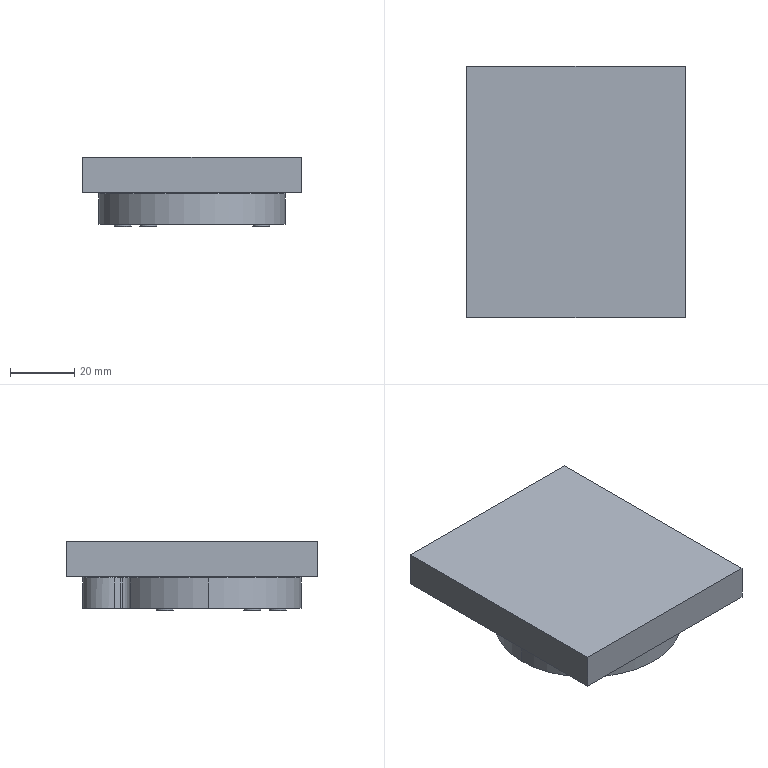NC program | NX | posted with a generic post | part box 68 x 78.27 x 21.8 mm
Lines 2834 to 3556 of 10371:
(CAVITY_MILL_COPY_COPY_COPY , TOOL : D2)
N5636 T17 M6
N5638 G54
N5640 G17 G0 G90 X1.507 Y24.709 S9500 M3
N5642 G43 Z30. H17
N5644 Z-0.5
N5646 G94 G1 Z-1. F1000.
N5648 G3 X0.772 Y24.654 R1.
N5650 G2 X0.207 Y24.506 R1.5 F2000.
N5652 G1 X-0.012 Y24.116
N5654 X-0.093 Y23.976
N5656 G3 X-0.189 Y23.149 R1.
N5658 G1 Z-0.5
N5660 G0 X1.507 Y24.709 Z-0.7
N5662 G1 Z-1.2 F1000.
N5664 G3 X0.772 Y24.654 R1.
N5666 G2 X0.207 Y24.506 R1.5 F2000.
N5668 G1 X-0.012 Y24.116
N5670 X-0.093 Y23.976
N5672 G3 X-0.189 Y23.149 R1.
N5674 G1 Z-0.7
N5676 G0 X1.507 Y24.709 Z-0.9
N5678 G1 Z-1.4 F1000.
N5680 G3 X0.772 Y24.654 R1.
N5682 G2 X0.207 Y24.506 R1.5 F2000.
N5684 G1 X-0.012 Y24.116
N5686 X-0.093 Y23.976
N5688 G3 X-0.189 Y23.149 R1.
N5690 G1 Z-0.9
N5692 G0 X1.507 Y24.709 Z-1.1
N5694 G1 Z-1.6 F1000.
N5696 G3 X0.772 Y24.654 R1.
N5698 G2 X0.207 Y24.506 R1.5 F2000.
N5700 G1 X-0.012 Y24.116
N5702 X-0.093 Y23.976
N5704 G3 X-0.189 Y23.149 R1.
N5706 G1 Z-1.1
N5708 G0 X1.507 Y24.709 Z-1.3
N5710 G1 Z-1.8 F1000.
N5712 G3 X0.772 Y24.654 R1.
N5714 G2 X0.207 Y24.506 R1.5 F2000.
N5716 G1 X-0.012 Y24.116
N5718 X-0.093 Y23.976
N5720 G3 X-0.189 Y23.149 R1.
N5722 G1 Z-1.3
N5724 G0 X1.507 Y24.709 Z-1.5
N5726 G1 Z-2. F1000.
N5728 G3 X0.772 Y24.654 R1.
N5730 G2 X0.207 Y24.506 R1.5 F2000.
N5732 G1 X-0.012 Y24.116
N5734 X-0.093 Y23.976
N5736 G3 X-0.189 Y23.149 R1.
N5738 G1 Z-1.5
N5740 G0 X1.507 Y24.709 Z-1.7
N5742 G1 Z-2.2 F1000.
N5744 G3 X0.772 Y24.654 R1.
N5746 G2 X0.207 Y24.506 R1.5 F2000.
N5748 G1 X-0.012 Y24.116
N5750 X-0.093 Y23.976
N5752 G3 X-0.189 Y23.149 R1.
N5754 G1 Z-1.7
N5756 G0 X1.507 Y24.709 Z-1.9
N5758 G1 Z-2.4 F1000.
N5760 G3 X0.772 Y24.654 R1.
N5762 G2 X0.207 Y24.506 R1.5 F2000.
N5764 G1 X-0.012 Y24.116
N5766 X-0.093 Y23.976
N5768 G3 X-0.189 Y23.149 R1.
N5770 G1 Z-1.9
N5772 G0 X1.507 Y24.709 Z-2.1
N5774 G1 Z-2.6 F1000.
N5776 G3 X0.772 Y24.654 R1.
N5778 G2 X0.207 Y24.506 R1.5 F2000.
N5780 G1 X-0.012 Y24.116
N5782 X-0.093 Y23.976
N5784 G3 X-0.189 Y23.149 R1.
N5786 G1 Z-2.1
N5788 G0 X1.507 Y24.709 Z-2.3
N5790 G1 Z-2.8 F1000.
N5792 G3 X0.772 Y24.654 R1.
N5794 G2 X0.207 Y24.506 R1.5 F2000.
N5796 G1 X-0.012 Y24.116
N5798 X-0.093 Y23.976
N5800 G3 X-0.189 Y23.149 R1.
N5802 G1 Z-2.3
N5804 G0 X1.507 Y24.709 Z-2.5
N5806 G1 Z-3. F1000.
N5808 G3 X0.772 Y24.654 R1.
N5810 G2 X0.207 Y24.506 R1.5 F2000.
N5812 G1 X-0.012 Y24.116
N5814 X-0.093 Y23.976
N5816 G3 X-0.189 Y23.149 R1.
N5818 G1 Z-2.5
N5820 G0 X1.507 Y24.709 Z-2.7
N5822 G1 Z-3.2 F1000.
N5824 G3 X0.772 Y24.654 R1.
N5826 G2 X0.207 Y24.506 R1.5 F2000.
N5828 G1 X-0.012 Y24.116
N5830 X-0.093 Y23.976
N5832 G3 X-0.189 Y23.149 R1.
N5834 G1 Z-2.7
N5836 G0 X1.507 Y24.709 Z-2.9
N5838 G1 Z-3.4 F1000.
N5840 G3 X0.772 Y24.654 R1.
N5842 G2 X0.207 Y24.506 R1.5 F2000.
N5844 G1 X-0.012 Y24.116
N5846 X-0.093 Y23.976
N5848 G3 X-0.189 Y23.149 R1.
N5850 G1 Z-2.9
N5852 G0 X1.507 Y24.709 Z-3.1
N5854 G1 Z-3.6 F1000.
N5856 G3 X0.772 Y24.654 R1.
N5858 G2 X0.207 Y24.506 R1.5 F2000.
N5860 G1 X-0.012 Y24.116
N5862 X-0.093 Y23.976
N5864 G3 X-0.189 Y23.149 R1.
N5866 G1 Z-3.1
N5868 G0 X1.507 Y24.709 Z-3.3
N5870 G1 Z-3.8 F1000.
N5872 G3 X0.772 Y24.654 R1.
N5874 G2 X0.207 Y24.506 R1.5 F2000.
N5876 G1 X-0.012 Y24.116
N5878 X-0.093 Y23.976
N5880 G3 X-0.189 Y23.149 R1.
N5882 G1 Z-3.3
N5884 G0 X1.507 Y24.709 Z-3.5
N5886 G1 Z-4. F1000.
N5888 G3 X0.772 Y24.654 R1.
N5890 G2 X0.207 Y24.506 R1.5 F2000.
N5892 G1 X-0.012 Y24.116
N5894 X-0.093 Y23.976
N5896 G3 X-0.189 Y23.149 R1.
N5898 G1 Z-3.5
N5900 G0 X1.507 Y24.709 Z-3.7
N5902 G1 Z-4.2 F1000.
N5904 G3 X0.772 Y24.654 R1.
N5906 G2 X0.207 Y24.506 R1.5 F2000.
N5908 G1 X-0.012 Y24.116
N5910 X-0.093 Y23.976
N5912 G3 X-0.189 Y23.149 R1.
N5914 G1 Z-3.7
N5916 G0 X1.507 Y24.709 Z-3.9
N5918 G1 Z-4.4 F1000.
N5920 G3 X0.772 Y24.654 R1.
N5922 G2 X0.207 Y24.506 R1.5 F2000.
N5924 G1 X-0.012 Y24.116
N5926 X-0.093 Y23.976
N5928 G3 X-0.189 Y23.149 R1.
N5930 G1 Z-3.9
N5932 G0 X1.507 Y24.709 Z-4.1
N5934 G1 Z-4.6 F1000.
N5936 G3 X0.772 Y24.654 R1.
N5938 G2 X0.207 Y24.506 R1.5 F2000.
N5940 G1 X-0.012 Y24.116
N5942 X-0.093 Y23.976
N5944 G3 X-0.189 Y23.149 R1.
N5946 G1 Z-4.1
N5948 G0 X1.507 Y24.709 Z-4.3
N5950 G1 Z-4.8 F1000.
N5952 G3 X0.772 Y24.654 R1.
N5954 G2 X0.207 Y24.506 R1.5 F2000.
N5956 G1 X-0.012 Y24.116
N5958 X-0.093 Y23.976
N5960 G3 X-0.189 Y23.149 R1.
N5962 G1 Z-4.3
N5964 G0 X1.507 Y24.709 Z-4.5
N5966 G1 Z-5. F1000.
N5968 G3 X0.772 Y24.654 R1.
N5970 G2 X0.207 Y24.506 R1.5 F2000.
N5972 G1 X-0.012 Y24.116
N5974 X-0.093 Y23.976
N5976 G3 X-0.189 Y23.149 R1.
N5978 G1 Z-4.5
N5980 G0 X1.507 Y24.709 Z-4.7
N5982 G1 Z-5.2 F1000.
N5984 G3 X0.772 Y24.654 R1.
N5986 G2 X0.207 Y24.506 R1.5 F2000.
N5988 G1 X-0.012 Y24.116
N5990 X-0.093 Y23.976
N5992 G3 X-0.189 Y23.149 R1.
N5994 G1 Z-4.7
N5996 G0 X1.507 Y24.709 Z-4.9
N5998 G1 Z-5.4 F1000.
N6000 G3 X0.772 Y24.654 R1.
N6002 G2 X0.207 Y24.506 R1.5 F2000.
N6004 G1 X-0.012 Y24.116
N6006 X-0.093 Y23.976
N6008 G3 X-0.189 Y23.149 R1.
N6010 G1 Z-4.9
N6012 G0 X1.507 Y24.709 Z-5.1
N6014 G1 Z-5.6 F1000.
N6016 G3 X0.772 Y24.654 R1.
N6018 G2 X0.207 Y24.506 R1.5 F2000.
N6020 G1 X-0.012 Y24.116
N6022 X-0.093 Y23.976
N6024 G3 X-0.189 Y23.149 R1.
N6026 G1 Z-5.1
N6028 G0 X1.507 Y24.709 Z-5.3
N6030 G1 Z-5.8 F1000.
N6032 G3 X0.772 Y24.654 R1.
N6034 G2 X0.207 Y24.506 R1.5 F2000.
N6036 G1 X-0.012 Y24.116
N6038 X-0.093 Y23.976
N6040 G3 X-0.189 Y23.149 R1.
N6042 G1 Z-5.3
N6044 G0 X1.507 Y24.709 Z-5.5
N6046 G1 Z-6. F1000.
N6048 G3 X0.772 Y24.654 R1.
N6050 G2 X0.207 Y24.506 R1.5 F2000.
N6052 G1 X-0.012 Y24.116
N6054 X-0.093 Y23.976
N6056 G3 X-0.189 Y23.149 R1.
N6058 G1 Z-5.5
N6060 G0 X1.507 Y24.709 Z-5.7
N6062 G1 Z-6.2 F1000.
N6064 G3 X0.772 Y24.654 R1.
N6066 G2 X0.207 Y24.506 R1.5 F2000.
N6068 G1 X-0.012 Y24.116
N6070 X-0.093 Y23.976
N6072 G3 X-0.189 Y23.149 R1.
N6074 G1 Z-5.7
N6076 G0 X1.507 Y24.709 Z-5.9
N6078 G1 Z-6.4 F1000.
N6080 G3 X0.772 Y24.654 R1.
N6082 G2 X0.207 Y24.506 R1.5 F2000.
N6084 G1 X-0.012 Y24.116
N6086 X-0.093 Y23.976
N6088 G3 X-0.189 Y23.149 R1.
N6090 G1 Z-5.9
N6092 G0 X1.507 Y24.709 Z-6.1
N6094 G1 Z-6.6 F1000.
N6096 G3 X0.772 Y24.654 R1.
N6098 G2 X0.207 Y24.506 R1.5 F2000.
N6100 G1 X-0.012 Y24.116
N6102 X-0.093 Y23.976
N6104 G3 X-0.189 Y23.149 R1.
N6106 G1 Z-6.1
N6108 G0 X1.507 Y24.709 Z-6.3
N6110 G1 Z-6.8 F1000.
N6112 G3 X0.772 Y24.654 R1.
N6114 G2 X0.207 Y24.506 R1.5 F2000.
N6116 G1 X-0.012 Y24.116
N6118 X-0.093 Y23.976
N6120 G3 X-0.189 Y23.149 R1.
N6122 G1 Z-6.3
N6124 G0 X1.507 Y24.709 Z-6.5
N6126 G1 Z-7. F1000.
N6128 G3 X0.772 Y24.654 R1.
N6130 G2 X0.207 Y24.506 R1.5 F2000.
N6132 G1 X-0.012 Y24.116
N6134 X-0.093 Y23.976
N6136 G3 X-0.189 Y23.149 R1.
N6138 G1 Z-6.5
N6140 G0 X1.507 Y24.709 Z-6.7
N6142 G1 Z-7.2 F1000.
N6144 G3 X0.772 Y24.654 R1.
N6146 G2 X0.207 Y24.506 R1.5 F2000.
N6148 G1 X-0.012 Y24.116
N6150 X-0.093 Y23.976
N6152 G3 X-0.189 Y23.149 R1.
N6154 G1 Z-6.7
N6156 G0 X1.507 Y24.709 Z-6.9
N6158 G1 Z-7.4 F1000.
N6160 G3 X0.772 Y24.654 R1.
N6162 G2 X0.207 Y24.506 R1.5 F2000.
N6164 G1 X-0.012 Y24.116
N6166 X-0.093 Y23.976
N6168 G3 X-0.189 Y23.149 R1.
N6170 G1 Z-6.9
N6172 G0 X1.507 Y24.709 Z-7.1
N6174 G1 Z-7.6 F1000.
N6176 G3 X0.772 Y24.654 R1.
N6178 G2 X0.207 Y24.506 R1.5 F2000.
N6180 G1 X-0.012 Y24.116
N6182 X-0.093 Y23.976
N6184 G3 X-0.189 Y23.149 R1.
N6186 G1 Z-7.1
N6188 G0 X1.507 Y24.709 Z-7.3
N6190 G1 Z-7.8 F1000.
N6192 G3 X0.772 Y24.654 R1.
N6194 G2 X0.207 Y24.506 R1.5 F2000.
N6196 G1 X-0.012 Y24.116
N6198 X-0.093 Y23.976
N6200 G3 X-0.189 Y23.149 R1.
N6202 G1 Z-7.3
N6204 G0 X1.507 Y24.709 Z-7.5
N6206 G1 Z-8. F1000.
N6208 G3 X0.772 Y24.654 R1.
N6210 G2 X0.207 Y24.506 R1.5 F2000.
N6212 G1 X-0.012 Y24.116
N6214 X-0.093 Y23.976
N6216 G3 X-0.189 Y23.149 R1.
N6218 G1 Z-7.5
N6220 G0 X1.507 Y24.709 Z-7.7
N6222 G1 Z-8.2 F1000.
N6224 G3 X0.772 Y24.654 R1.
N6226 G2 X0.207 Y24.506 R1.5 F2000.
N6228 G1 X-0.012 Y24.116
N6230 X-0.093 Y23.976
N6232 G3 X-0.189 Y23.149 R1.
N6234 G1 Z-7.7
N6236 G0 X1.507 Y24.709 Z-7.9
N6238 G1 Z-8.4 F1000.
N6240 G3 X0.772 Y24.654 R1.
N6242 G2 X0.207 Y24.506 R1.5 F2000.
N6244 G1 X-0.012 Y24.116
N6246 X-0.093 Y23.976
N6248 G3 X-0.189 Y23.149 R1.
N6250 G1 Z-7.9
N6252 G0 X1.507 Y24.709 Z-8.1
N6254 G1 Z-8.6 F1000.
N6256 G3 X0.772 Y24.654 R1.
N6258 G2 X0.207 Y24.506 R1.5 F2000.
N6260 G1 X-0.012 Y24.116
N6262 X-0.093 Y23.976
N6264 G3 X-0.189 Y23.149 R1.
N6266 G1 Z-8.1
N6268 G0 X1.507 Y24.709 Z-8.3
N6270 G1 Z-8.8 F1000.
N6272 G3 X0.772 Y24.654 R1.
N6274 G2 X0.207 Y24.506 R1.5 F2000.
N6276 G1 X-0.012 Y24.116
N6278 X-0.093 Y23.976
N6280 G3 X-0.189 Y23.149 R1.
N6282 G1 Z-8.3
N6284 G0 X1.764 Y23.744 Z-8.5
N6286 G1 Z-9. F1000.
N6288 G3 X1.071 Y24.31 R1.
N6290 G1 X0.207 Y24.506 F2000.
N6292 X-0.012 Y24.116
N6294 G2 X-0.237 Y23.752 R5.
N6296 G3 X-0.377 Y22.931 R1.
N6298 G1 Z-8.5
N6300 G0 X1.764 Y23.744 Z-8.7
N6302 G1 Z-9.2 F1000.
N6304 G3 X1.071 Y24.31 R1.
N6306 G1 X0.207 Y24.506 F2000.
N6308 X-0.012 Y24.116
N6310 G2 X-0.237 Y23.752 R5.
N6312 G3 X-0.377 Y22.931 R1.
N6314 G1 Z-8.7
N6316 G0 X1.764 Y23.744 Z-8.9
N6318 G1 Z-9.4 F1000.
N6320 G3 X1.071 Y24.31 R1.
N6322 G1 X0.207 Y24.506 F2000.
N6324 X-0.012 Y24.116
N6326 G2 X-0.237 Y23.752 R5.
N6328 G3 X-0.377 Y22.931 R1.
N6330 G1 Z-8.9
N6332 G0 X1.764 Y23.744 Z-9.1
N6334 G1 Z-9.6 F1000.
N6336 G3 X1.071 Y24.31 R1.
N6338 G1 X0.207 Y24.506 F2000.
N6340 X-0.012 Y24.116
N6342 G2 X-0.237 Y23.752 R5.
N6344 G3 X-0.377 Y22.931 R1.
N6346 G1 Z-9.1
N6348 G0 X1.764 Y23.744 Z-9.3
N6350 G1 Z-9.8 F1000.
N6352 G3 X1.071 Y24.31 R1.
N6354 G1 X0.207 Y24.506 F2000.
N6356 X-0.012 Y24.116
N6358 G2 X-0.237 Y23.752 R5.
N6360 G3 X-0.377 Y22.931 R1.
N6362 G1 Z-9.3
N6364 G0 Z-5.8
N6366 X11.299 Y20.207
N6368 Z-8.5
N6370 G1 Z-9. F1000.
N6372 G3 X11.604 Y21.027 R1.
N6374 G2 X11.576 Y21.59 R6. F2000.
N6376 G3 X10.947 Y22.079 R1.
N6378 X10.051 Y21.871 R1.
N6380 G1 Z-8.5
N6382 G0 X11.299 Y20.207 Z-8.7
N6384 G1 Z-9.2 F1000.
N6386 G3 X11.604 Y21.027 R1.
N6388 G2 X11.576 Y21.59 R6. F2000.
N6390 G3 X10.947 Y22.079 R1.
N6392 X10.051 Y21.871 R1.
N6394 G1 Z-8.7
N6396 G0 X11.299 Y20.207 Z-8.9
N6398 G1 Z-9.4 F1000.
N6400 G3 X11.604 Y21.027 R1.
N6402 G2 X11.576 Y21.59 R6. F2000.
N6404 G3 X10.947 Y22.079 R1.
N6406 X10.051 Y21.871 R1.
N6408 G1 Z-8.9
N6410 G0 X11.299 Y20.207 Z-9.1
N6412 G1 Z-9.6 F1000.
N6414 G3 X11.604 Y21.027 R1.
N6416 G2 X11.576 Y21.59 R6. F2000.
N6418 G3 X10.947 Y22.079 R1.
N6420 X10.051 Y21.871 R1.
N6422 G1 Z-9.1
N6424 G0 X11.299 Y20.207 Z-9.3
N6426 G1 Z-9.8 F1000.
N6428 G3 X11.604 Y21.027 R1.
N6430 G2 X11.576 Y21.59 R6. F2000.
N6432 G3 X10.947 Y22.079 R1.
N6434 X10.051 Y21.871 R1.
N6436 G1 Z-9.3
N6438 G0 Z30.
N6440 X-15.708 Y16.332
N6442 Z-0.5
N6444 G1 Z-1. F1000.
N6446 G3 X-16.599 Y16.16 R1.
N6448 X-17.192 Y15.684 R27. F2000.
N6450 G2 X-17.093 Y14.996 R1.5
N6452 G3 X-16.885 Y14.288 R1.
N6454 G1 Z-0.5
N6456 G0 X-15.708 Y16.332 Z-0.7
N6458 G1 Z-1.2 F1000.
N6460 G3 X-16.599 Y16.16 R1.
N6462 X-17.192 Y15.684 R27. F2000.
N6464 G2 X-17.093 Y14.996 R1.5
N6466 G3 X-16.885 Y14.288 R1.
N6468 G1 Z-0.7
N6470 G0 X-15.708 Y16.332 Z-0.9
N6472 G1 Z-1.4 F1000.
N6474 G3 X-16.599 Y16.16 R1.
N6476 X-17.192 Y15.684 R27. F2000.
N6478 G2 X-17.093 Y14.996 R1.5
N6480 G3 X-16.885 Y14.288 R1.
N6482 G1 Z-0.9
N6484 G0 X-15.708 Y16.332 Z-1.1
N6486 G1 Z-1.6 F1000.
N6488 G3 X-16.599 Y16.16 R1.
N6490 X-17.192 Y15.684 R27. F2000.
N6492 G2 X-17.093 Y14.996 R1.5
N6494 G3 X-16.885 Y14.288 R1.
N6496 G1 Z-1.1
N6498 G0 X-15.708 Y16.332 Z-1.3
N6500 G1 Z-1.8 F1000.
N6502 G3 X-16.599 Y16.16 R1.
N6504 X-17.192 Y15.684 R27. F2000.
N6506 G2 X-17.093 Y14.996 R1.5
N6508 G3 X-16.885 Y14.288 R1.
N6510 G1 Z-1.3
N6512 G0 X-15.708 Y16.332 Z-1.5
N6514 G1 Z-2. F1000.
N6516 G3 X-16.599 Y16.16 R1.
N6518 X-17.192 Y15.684 R27. F2000.
N6520 G2 X-17.093 Y14.996 R1.5
N6522 G3 X-16.885 Y14.288 R1.
N6524 G1 Z-1.5
N6526 G0 X-15.708 Y16.332 Z-1.7
N6528 G1 Z-2.2 F1000.
N6530 G3 X-16.599 Y16.16 R1.
N6532 X-17.192 Y15.684 R27. F2000.
N6534 G2 X-17.093 Y14.996 R1.5
N6536 G3 X-16.885 Y14.288 R1.
N6538 G1 Z-1.7
N6540 G0 X-15.708 Y16.332 Z-1.9
N6542 G1 Z-2.4 F1000.
N6544 G3 X-16.599 Y16.16 R1.
N6546 X-17.192 Y15.684 R27. F2000.
N6548 G2 X-17.093 Y14.996 R1.5
N6550 G3 X-16.885 Y14.288 R1.
N6552 G1 Z-1.9
N6554 G0 X-15.708 Y16.332 Z-2.1
N6556 G1 Z-2.6 F1000.
N6558 G3 X-16.599 Y16.16 R1.
N6560 X-17.192 Y15.684 R27. F2000.
N6562 G2 X-17.093 Y14.996 R1.5
N6564 G3 X-16.885 Y14.288 R1.
N6566 G1 Z-2.1
N6568 G0 X-15.708 Y16.332 Z-2.3
N6570 G1 Z-2.8 F1000.
N6572 G3 X-16.599 Y16.16 R1.
N6574 X-17.192 Y15.684 R27. F2000.
N6576 G2 X-17.093 Y14.996 R1.5
N6578 G3 X-16.885 Y14.288 R1.
N6580 G1 Z-2.3
N6582 G0 X-15.708 Y16.332 Z-2.5
N6584 G1 Z-3. F1000.
N6586 G3 X-16.599 Y16.16 R1.
N6588 X-17.192 Y15.684 R27. F2000.
N6590 G2 X-17.093 Y14.996 R1.5
N6592 G3 X-16.885 Y14.288 R1.
N6594 G1 Z-2.5
N6596 G0 X-15.708 Y16.332 Z-2.7
N6598 G1 Z-3.2 F1000.
N6600 G3 X-16.599 Y16.16 R1.
N6602 X-17.192 Y15.684 R27. F2000.
N6604 G2 X-17.093 Y14.996 R1.5
N6606 G3 X-16.885 Y14.288 R1.
N6608 G1 Z-2.7
N6610 G0 X-15.708 Y16.332 Z-2.9
N6612 G1 Z-3.4 F1000.
N6614 G3 X-16.599 Y16.16 R1.
N6616 X-17.192 Y15.684 R27. F2000.
N6618 G2 X-17.093 Y14.996 R1.5
N6620 G3 X-16.885 Y14.288 R1.
N6622 G1 Z-2.9
N6624 G0 X-15.708 Y16.332 Z-3.1
N6626 G1 Z-3.6 F1000.
N6628 G3 X-16.599 Y16.16 R1.
N6630 X-17.192 Y15.684 R27. F2000.
N6632 G2 X-17.093 Y14.996 R1.5
N6634 G3 X-16.885 Y14.288 R1.
N6636 G1 Z-3.1
N6638 G0 X-15.708 Y16.332 Z-3.3
N6640 G1 Z-3.8 F1000.
N6642 G3 X-16.599 Y16.16 R1.
N6644 X-17.192 Y15.684 R27. F2000.
N6646 G2 X-17.093 Y14.996 R1.5
N6648 G3 X-16.885 Y14.288 R1.
N6650 G1 Z-3.3
N6652 G0 X-15.708 Y16.332 Z-3.5
N6654 G1 Z-4. F1000.
N6656 G3 X-16.599 Y16.16 R1.
N6658 X-17.192 Y15.684 R27. F2000.
N6660 G2 X-17.093 Y14.996 R1.5
N6662 G3 X-16.885 Y14.288 R1.
N6664 G1 Z-3.5
N6666 G0 X-15.708 Y16.332 Z-3.7
N6668 G1 Z-4.2 F1000.
N6670 G3 X-16.599 Y16.16 R1.
N6672 X-17.192 Y15.684 R27. F2000.
N6674 G2 X-17.093 Y14.996 R1.5
N6676 G3 X-16.885 Y14.288 R1.
N6678 G1 Z-3.7
N6680 G0 X-15.708 Y16.332 Z-3.9
N6682 G1 Z-4.4 F1000.
N6684 G3 X-16.599 Y16.16 R1.
N6686 X-17.192 Y15.684 R27. F2000.
N6688 G2 X-17.093 Y14.996 R1.5
N6690 G3 X-16.885 Y14.288 R1.
N6692 G1 Z-3.9
N6694 G0 X-15.708 Y16.332 Z-4.1
N6696 G1 Z-4.6 F1000.
N6698 G3 X-16.599 Y16.16 R1.
N6700 X-17.192 Y15.684 R27. F2000.
N6702 G2 X-17.093 Y14.996 R1.5
N6704 G3 X-16.885 Y14.288 R1.
N6706 G1 Z-4.1
N6708 G0 X-15.708 Y16.332 Z-4.3
N6710 G1 Z-4.8 F1000.
N6712 G3 X-16.599 Y16.16 R1.
N6714 X-17.192 Y15.684 R27. F2000.
N6716 G2 X-17.093 Y14.996 R1.5
N6718 G3 X-16.885 Y14.288 R1.
N6720 G1 Z-4.3
N6722 G0 X-15.708 Y16.332 Z-4.5
N6724 G1 Z-5. F1000.
N6726 G3 X-16.599 Y16.16 R1.
N6728 X-17.192 Y15.684 R27. F2000.
N6730 G2 X-17.093 Y14.996 R1.5
N6732 G3 X-16.885 Y14.288 R1.
N6734 G1 Z-4.5
N6736 G0 X-15.708 Y16.332 Z-4.7
N6738 G1 Z-5.2 F1000.
N6740 G3 X-16.599 Y16.16 R1.
N6742 X-17.192 Y15.684 R27. F2000.
N6744 G2 X-17.093 Y14.996 R1.5
N6746 G3 X-16.885 Y14.288 R1.
N6748 G1 Z-4.7
N6750 G0 X-15.708 Y16.332 Z-4.9
N6752 G1 Z-5.4 F1000.
N6754 G3 X-16.599 Y16.16 R1.
N6756 X-17.192 Y15.684 R27. F2000.
N6758 G2 X-17.093 Y14.996 R1.5
N6760 G3 X-16.885 Y14.288 R1.
N6762 G1 Z-4.9
N6764 G0 X-15.708 Y16.332 Z-5.1
N6766 G1 Z-5.6 F1000.
N6768 G3 X-16.599 Y16.16 R1.
N6770 X-17.192 Y15.684 R27. F2000.
N6772 G2 X-17.093 Y14.996 R1.5
N6774 G3 X-16.885 Y14.288 R1.
N6776 G1 Z-5.1
N6778 G0 X-15.708 Y16.332 Z-5.3
N6780 G1 Z-5.8 F1000.
N6782 G3 X-16.599 Y16.16 R1.
N6784 X-17.192 Y15.684 R27. F2000.
N6786 G2 X-17.093 Y14.996 R1.5
N6788 G3 X-16.885 Y14.288 R1.
N6790 G1 Z-5.3
N6792 G0 X-15.708 Y16.332 Z-5.5
N6794 G1 Z-6. F1000.
N6796 G3 X-16.599 Y16.16 R1.
N6798 X-17.192 Y15.684 R27. F2000.
N6800 G2 X-17.093 Y14.996 R1.5
N6802 G3 X-16.885 Y14.288 R1.
N6804 G1 Z-5.5
N6806 G0 X-15.708 Y16.332 Z-5.7
N6808 G1 Z-6.2 F1000.
N6810 G3 X-16.599 Y16.16 R1.
N6812 X-17.192 Y15.684 R27. F2000.
N6814 G2 X-17.093 Y14.996 R1.5
N6816 G3 X-16.885 Y14.288 R1.
N6818 G1 Z-5.7
N6820 G0 X-15.708 Y16.332 Z-5.9
N6822 G1 Z-6.4 F1000.
N6824 G3 X-16.599 Y16.16 R1.
N6826 X-17.192 Y15.684 R27. F2000.
N6828 G2 X-17.093 Y14.996 R1.5
N6830 G3 X-16.885 Y14.288 R1.
N6832 G1 Z-5.9
N6834 G0 X-15.708 Y16.332 Z-6.1
N6836 G1 Z-6.6 F1000.
N6838 G3 X-16.599 Y16.16 R1.
N6840 X-17.192 Y15.684 R27. F2000.
N6842 G2 X-17.093 Y14.996 R1.5
N6844 G3 X-16.885 Y14.288 R1.
N6846 G1 Z-6.1
N6848 G0 X-15.708 Y16.332 Z-6.3
N6850 G1 Z-6.8 F1000.
N6852 G3 X-16.599 Y16.16 R1.
N6854 X-17.192 Y15.684 R27. F2000.
N6856 G2 X-17.093 Y14.996 R1.5
N6858 G3 X-16.885 Y14.288 R1.
N6860 G1 Z-6.3
N6862 G0 X-15.708 Y16.332 Z-6.5
N6864 G1 Z-7. F1000.
N6866 G3 X-16.599 Y16.16 R1.
N6868 X-17.192 Y15.684 R27. F2000.
N6870 G2 X-17.093 Y14.996 R1.5
N6872 G3 X-16.885 Y14.288 R1.
N6874 G1 Z-6.5
N6876 G0 X-15.708 Y16.332 Z-6.7
N6878 G1 Z-7.2 F1000.
N6880 G3 X-16.599 Y16.16 R1.
N6882 X-17.192 Y15.684 R27. F2000.
N6884 G2 X-17.093 Y14.996 R1.5
N6886 G3 X-16.885 Y14.288 R1.
N6888 G1 Z-6.7
N6890 G0 X-15.708 Y16.332 Z-6.9
N6892 G1 Z-7.4 F1000.
N6894 G3 X-16.599 Y16.16 R1.
N6896 X-17.192 Y15.684 R27. F2000.
N6898 G2 X-17.093 Y14.996 R1.5
N6900 G3 X-16.885 Y14.288 R1.
N6902 G1 Z-6.9
N6904 G0 X-15.708 Y16.332 Z-7.1
N6906 G1 Z-7.6 F1000.
N6908 G3 X-16.599 Y16.16 R1.
N6910 X-17.192 Y15.684 R27. F2000.
N6912 G2 X-17.093 Y14.996 R1.5
N6914 G3 X-16.885 Y14.288 R1.
N6916 G1 Z-7.1
N6918 G0 X-15.708 Y16.332 Z-7.3
N6920 G1 Z-7.8 F1000.
N6922 G3 X-16.599 Y16.16 R1.
N6924 X-17.192 Y15.684 R27. F2000.
N6926 G2 X-17.093 Y14.996 R1.5
N6928 G3 X-16.885 Y14.288 R1.
N6930 G1 Z-7.3
N6932 G0 X-15.708 Y16.332 Z-7.5
N6934 G1 Z-8. F1000.
N6936 G3 X-16.599 Y16.16 R1.
N6938 X-17.192 Y15.684 R27. F2000.
N6940 G2 X-17.093 Y14.996 R1.5
N6942 G3 X-16.885 Y14.288 R1.
N6944 G1 Z-7.5
N6946 G0 X-15.708 Y16.332 Z-7.7
N6948 G1 Z-8.2 F1000.
N6950 G3 X-16.599 Y16.16 R1.
N6952 X-17.192 Y15.684 R27. F2000.
N6954 G2 X-17.093 Y14.996 R1.5
N6956 G3 X-16.885 Y14.288 R1.
N6958 G1 Z-7.7
N6960 G0 X-15.708 Y16.332 Z-7.9
N6962 G1 Z-8.4 F1000.
N6964 G3 X-16.599 Y16.16 R1.
N6966 X-17.192 Y15.684 R27. F2000.
N6968 G2 X-17.093 Y14.996 R1.5
N6970 G3 X-16.885 Y14.288 R1.
N6972 G1 Z-7.9
N6974 G0 X-15.708 Y16.332 Z-8.1
N6976 G1 Z-8.6 F1000.
N6978 G3 X-16.599 Y16.16 R1.
N6980 X-17.192 Y15.684 R27. F2000.
N6982 G2 X-17.093 Y14.996 R1.5
N6984 G3 X-16.885 Y14.288 R1.
N6986 G1 Z-8.1
N6988 G0 X-15.708 Y16.332 Z-8.3
N6990 G1 Z-8.8 F1000.
N6992 G3 X-16.599 Y16.16 R1.
N6994 X-17.192 Y15.684 R27. F2000.
N6996 G2 X-17.093 Y14.996 R1.5
N6998 G3 X-16.885 Y14.288 R1.
N7000 G1 Z-8.3
N7002 G0 X-15.467 Y16.506 Z-8.5
N7004 G1 Z-9. F1000.
N7006 G3 X-16.361 Y16.344 R1.
N7008 X-17.192 Y15.684 R27. F2000.
N7010 G1 X-16.624 Y14.8
N7012 G3 X-15.856 Y14.343 R1.
N7014 G1 Z-8.5
N7016 G0 X-15.467 Y16.506 Z-8.7
N7018 G1 Z-9.2 F1000.
N7020 G3 X-16.361 Y16.344 R1.
N7022 X-17.192 Y15.684 R27. F2000.
N7024 G1 X-16.624 Y14.8
N7026 G3 X-15.856 Y14.343 R1.
N7028 G1 Z-8.7
N7030 G0 X-15.467 Y16.506 Z-8.9
N7032 G1 Z-9.4 F1000.
N7034 G3 X-16.361 Y16.344 R1.
N7036 X-17.192 Y15.684 R27. F2000.
N7038 G1 X-16.624 Y14.8
N7040 G3 X-15.856 Y14.343 R1.
N7042 G1 Z-8.9
N7044 G0 X-15.467 Y16.506 Z-9.1
N7046 G1 Z-9.6 F1000.
N7048 G3 X-16.361 Y16.344 R1.
N7050 X-17.192 Y15.684 R27. F2000.
N7052 G1 X-16.624 Y14.8
N7054 G3 X-15.856 Y14.343 R1.
N7056 G1 Z-9.1
N7058 G0 X-15.467 Y16.506 Z-9.3
N7060 G1 Z-9.8 F1000.
N7062 G3 X-16.361 Y16.344 R1.
N7064 X-17.192 Y15.684 R27. F2000.
N7066 G1 X-16.624 Y14.8
N7068 G3 X-15.856 Y14.343 R1.
N7070 G1 Z-9.3
N7072 G0 Z30.
N7074 M5